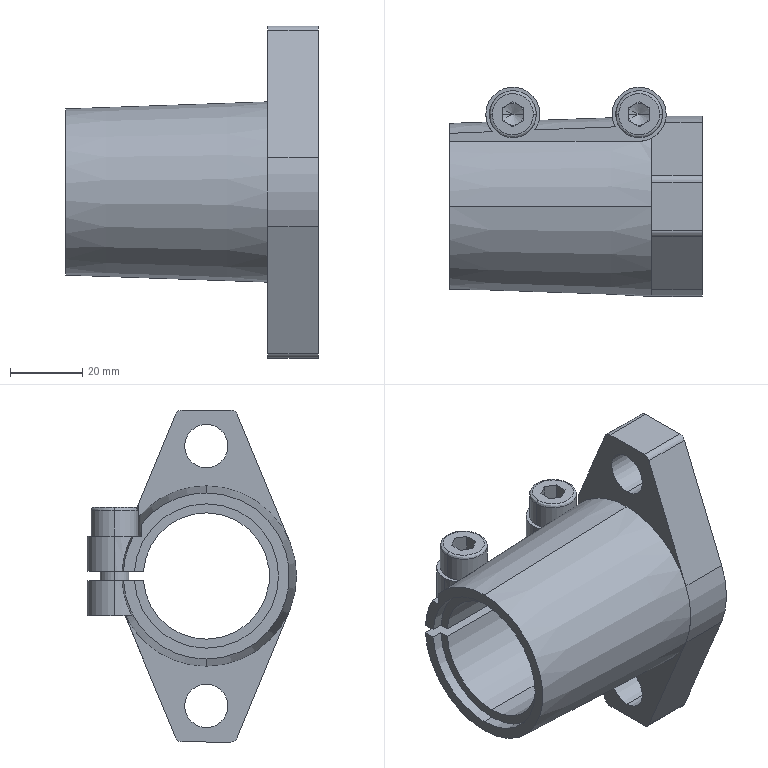Part | SolidWorks | features BaseBody 3 | 3 solids | 138 faces | box 70 x 58 x 92 mm | volume 80173 mm3 | cylinder 47 | plane 46 | cone 33 | spline 12 | commonest cylinder face diameters 15 x13 6.647 x8 8 x5 4 x4 12 x4 13 x4